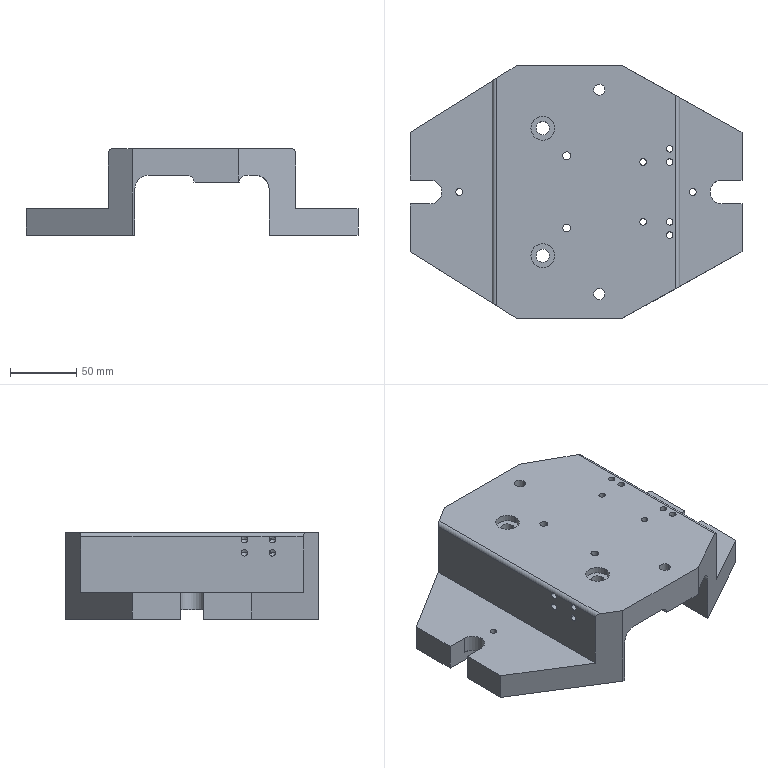Part | SolidWorks | features ICE 10, MoveFace 2, BaseBody 1, Cut 1 | 1 solid | 95 faces | box 250 x 190 x 65 mm | volume 1073575 mm3 | cylinder 53 | plane 34 | cone 8 | commonest cylinder face diameters 5 x24 18 x7 6 x6 10 x6 8.5 x4 12 x4